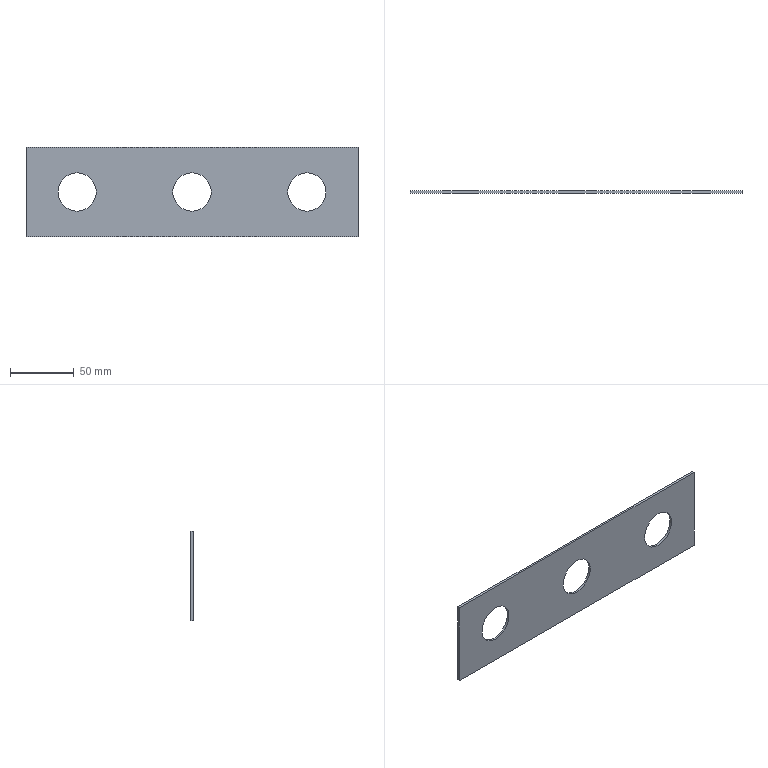Part | STEP file | tutup bawah | 1 solid | 12 faces | box 260 x 1.8 x 70 mm | volume 28943 mm3 | cylinder 6 | plane 6 | commonest cylinder face diameters 30 x6
STEP:
#1=CARTESIAN_POINT('',(0.,0.,0.));
#2=DIRECTION('',(0.,0.,1.));
#3=DIRECTION('',(1.,0.,0.));
#4=AXIS2_PLACEMENT_3D('',#1,#2,#3);
#5=CARTESIAN_POINT('',(90.,1.8,-15.));
#6=VERTEX_POINT('',#5);
#7=CARTESIAN_POINT('',(90.,0.,-15.));
#8=VERTEX_POINT('',#7);
#9=CARTESIAN_POINT('',(90.,1.8,-15.));
#10=DIRECTION('',(0.,-1.,0.));
#11=VECTOR('',#10,1.);
#12=LINE('',#9,#11);
#13=CARTESIAN_POINT('',(90.,1.8,0.));
#14=DIRECTION('',(0.,-1.,0.));
#15=DIRECTION('',(0.,0.,-1.));
#16=AXIS2_PLACEMENT_3D('',#13,#14,#15);
#17=CYLINDRICAL_SURFACE('',#16,15.);
#18=CARTESIAN_POINT('',(6.283,0.));
#19=DIRECTION('',(0.,1.));
#20=VECTOR('',#19,1.);
#21=LINE('',#18,#20);
#22=(GEOMETRIC_REPRESENTATION_CONTEXT(2)PARAMETRIC_REPRESENTATION_CONTEXT()REPRESENTATION_CONTEXT('',''));
#23=DEFINITIONAL_REPRESENTATION('',(#21),#22);
#24=PCURVE('',#17,#23);
#25=CARTESIAN_POINT('',(90.,1.8,0.));
#26=DIRECTION('',(0.,-1.,0.));
#27=DIRECTION('',(0.,0.,-1.));
#28=AXIS2_PLACEMENT_3D('',#25,#26,#27);
#29=CYLINDRICAL_SURFACE('',#28,15.);
#30=CARTESIAN_POINT('',(0.,0.));
#31=DIRECTION('',(0.,1.));
#32=VECTOR('',#31,1.);
#33=LINE('',#30,#32);
#34=(GEOMETRIC_REPRESENTATION_CONTEXT(2)PARAMETRIC_REPRESENTATION_CONTEXT()REPRESENTATION_CONTEXT('',''));
#35=DEFINITIONAL_REPRESENTATION('',(#33),#34);
#36=PCURVE('',#29,#35);
#37=SURFACE_CURVE('',#12,(#24,#36),.PCURVE_S1.);
#38=EDGE_CURVE('',#6,#8,#37,.T.);
#39=ORIENTED_EDGE('',*,*,#38,.T.);
#40=CARTESIAN_POINT('',(90.,0.,15.));
#41=VERTEX_POINT('',#40);
#42=CARTESIAN_POINT('',(90.,0.,0.));
#43=DIRECTION('',(0.,1.,0.));
#44=DIRECTION('',(0.,0.,-1.));
#45=AXIS2_PLACEMENT_3D('',#42,#43,#44);
#46=CIRCLE('',#45,15.);
#47=CARTESIAN_POINT('',(6.283,1.8));
#48=DIRECTION('',(-1.,0.));
#49=VECTOR('',#48,1.);
#50=LINE('',#47,#49);
#51=(GEOMETRIC_REPRESENTATION_CONTEXT(2)PARAMETRIC_REPRESENTATION_CONTEXT()REPRESENTATION_CONTEXT('',''));
#52=DEFINITIONAL_REPRESENTATION('',(#50),#51);
#53=PCURVE('',#17,#52);
#54=CARTESIAN_POINT('',(130.,0.,35.));
#55=DIRECTION('',(0.,1.,0.));
#56=DIRECTION('',(0.,0.,1.));
#57=AXIS2_PLACEMENT_3D('',#54,#55,#56);
#58=PLANE('',#57);
#59=CARTESIAN_POINT('',(-35.,-40.));
#60=DIRECTION('',(-1.,0.));
#61=AXIS2_PLACEMENT_2D('',#59,#60);
#62=CIRCLE('',#61,15.);
#63=(GEOMETRIC_REPRESENTATION_CONTEXT(2)PARAMETRIC_REPRESENTATION_CONTEXT()REPRESENTATION_CONTEXT('',''));
#64=DEFINITIONAL_REPRESENTATION('',(#62),#63);
#65=PCURVE('',#58,#64);
#66=SURFACE_CURVE('',#46,(#53,#65),.PCURVE_S1.);
#67=EDGE_CURVE('',#8,#41,#66,.T.);
#68=ORIENTED_EDGE('',*,*,#67,.T.);
#69=CARTESIAN_POINT('',(90.,1.8,15.));
#70=VERTEX_POINT('',#69);
#71=CARTESIAN_POINT('',(90.,1.8,15.));
#72=DIRECTION('',(0.,-1.,0.));
#73=VECTOR('',#72,1.);
#74=LINE('',#71,#73);
#75=CARTESIAN_POINT('',(3.142,0.));
#76=DIRECTION('',(0.,1.));
#77=VECTOR('',#76,1.);
#78=LINE('',#75,#77);
#79=(GEOMETRIC_REPRESENTATION_CONTEXT(2)PARAMETRIC_REPRESENTATION_CONTEXT()REPRESENTATION_CONTEXT('',''));
#80=DEFINITIONAL_REPRESENTATION('',(#78),#79);
#81=PCURVE('',#17,#80);
#82=CARTESIAN_POINT('',(3.142,0.));
#83=DIRECTION('',(0.,1.));
#84=VECTOR('',#83,1.);
#85=LINE('',#82,#84);
#86=(GEOMETRIC_REPRESENTATION_CONTEXT(2)PARAMETRIC_REPRESENTATION_CONTEXT()REPRESENTATION_CONTEXT('',''));
#87=DEFINITIONAL_REPRESENTATION('',(#85),#86);
#88=PCURVE('',#29,#87);
#89=SURFACE_CURVE('',#74,(#81,#88),.PCURVE_S1.);
#90=EDGE_CURVE('',#70,#41,#89,.T.);
#91=ORIENTED_EDGE('',*,*,#90,.F.);
#92=CARTESIAN_POINT('',(90.,1.8,0.));
#93=DIRECTION('',(0.,1.,0.));
#94=DIRECTION('',(0.,0.,-1.));
#95=AXIS2_PLACEMENT_3D('',#92,#93,#94);
#96=CIRCLE('',#95,15.);
#97=CARTESIAN_POINT('',(6.283,0.));
#98=DIRECTION('',(-1.,0.));
#99=VECTOR('',#98,1.);
#100=LINE('',#97,#99);
#101=(GEOMETRIC_REPRESENTATION_CONTEXT(2)PARAMETRIC_REPRESENTATION_CONTEXT()REPRESENTATION_CONTEXT('',''));
#102=DEFINITIONAL_REPRESENTATION('',(#100),#101);
#103=PCURVE('',#17,#102);
#104=CARTESIAN_POINT('',(130.,1.8,35.));
#105=DIRECTION('',(0.,1.,0.));
#106=DIRECTION('',(0.,0.,1.));
#107=AXIS2_PLACEMENT_3D('',#104,#105,#106);
#108=PLANE('',#107);
#109=CARTESIAN_POINT('',(-35.,-40.));
#110=DIRECTION('',(-1.,0.));
#111=AXIS2_PLACEMENT_2D('',#109,#110);
#112=CIRCLE('',#111,15.);
#113=(GEOMETRIC_REPRESENTATION_CONTEXT(2)PARAMETRIC_REPRESENTATION_CONTEXT()REPRESENTATION_CONTEXT('',''));
#114=DEFINITIONAL_REPRESENTATION('',(#112),#113);
#115=PCURVE('',#108,#114);
#116=SURFACE_CURVE('',#96,(#103,#115),.PCURVE_S1.);
#117=EDGE_CURVE('',#6,#70,#116,.T.);
#118=ORIENTED_EDGE('',*,*,#117,.F.);
#119=EDGE_LOOP('',(#39,#68,#91,#118));
#120=FACE_BOUND('',#119,.F.);
#121=ADVANCED_FACE('',(#120),#17,.F.);
#122=CARTESIAN_POINT('',(0.,1.8,-15.));
#123=VERTEX_POINT('',#122);
#124=CARTESIAN_POINT('',(0.,0.,-15.));
#125=VERTEX_POINT('',#124);
#126=CARTESIAN_POINT('',(0.,1.8,-15.));
#127=DIRECTION('',(0.,-1.,0.));
#128=VECTOR('',#127,1.);
#129=LINE('',#126,#128);
#130=CARTESIAN_POINT('',(0.,1.8,0.));
#131=DIRECTION('',(0.,-1.,0.));
#132=DIRECTION('',(0.,0.,-1.));
#133=AXIS2_PLACEMENT_3D('',#130,#131,#132);
#134=CYLINDRICAL_SURFACE('',#133,15.);
#135=CARTESIAN_POINT('',(6.283,0.));
#136=DIRECTION('',(0.,1.));
#137=VECTOR('',#136,1.);
#138=LINE('',#135,#137);
#139=(GEOMETRIC_REPRESENTATION_CONTEXT(2)PARAMETRIC_REPRESENTATION_CONTEXT()REPRESENTATION_CONTEXT('',''));
#140=DEFINITIONAL_REPRESENTATION('',(#138),#139);
#141=PCURVE('',#134,#140);
#142=CARTESIAN_POINT('',(0.,1.8,0.));
#143=DIRECTION('',(0.,-1.,0.));
#144=DIRECTION('',(0.,0.,-1.));
#145=AXIS2_PLACEMENT_3D('',#142,#143,#144);
#146=CYLINDRICAL_SURFACE('',#145,15.);
#147=CARTESIAN_POINT('',(0.,0.));
#148=DIRECTION('',(0.,1.));
#149=VECTOR('',#148,1.);
#150=LINE('',#147,#149);
#151=(GEOMETRIC_REPRESENTATION_CONTEXT(2)PARAMETRIC_REPRESENTATION_CONTEXT()REPRESENTATION_CONTEXT('',''));
#152=DEFINITIONAL_REPRESENTATION('',(#150),#151);
#153=PCURVE('',#146,#152);
#154=SURFACE_CURVE('',#129,(#141,#153),.PCURVE_S1.);
#155=EDGE_CURVE('',#123,#125,#154,.T.);
#156=ORIENTED_EDGE('',*,*,#155,.T.);
#157=CARTESIAN_POINT('',(0.,0.,15.));
#158=VERTEX_POINT('',#157);
#159=CARTESIAN_POINT('',(0.,0.,0.));
#160=DIRECTION('',(0.,1.,0.));
#161=DIRECTION('',(0.,0.,1.));
#162=AXIS2_PLACEMENT_3D('',#159,#160,#161);
#163=CIRCLE('',#162,15.);
#164=CARTESIAN_POINT('',(9.425,1.8));
#165=DIRECTION('',(-1.,0.));
#166=VECTOR('',#165,1.);
#167=LINE('',#164,#166);
#168=(GEOMETRIC_REPRESENTATION_CONTEXT(2)PARAMETRIC_REPRESENTATION_CONTEXT()REPRESENTATION_CONTEXT('',''));
#169=DEFINITIONAL_REPRESENTATION('',(#167),#168);
#170=PCURVE('',#134,#169);
#171=CARTESIAN_POINT('',(-35.,-130.));
#172=DIRECTION('',(1.,0.));
#173=AXIS2_PLACEMENT_2D('',#171,#172);
#174=CIRCLE('',#173,15.);
#175=(GEOMETRIC_REPRESENTATION_CONTEXT(2)PARAMETRIC_REPRESENTATION_CONTEXT()REPRESENTATION_CONTEXT('',''));
#176=DEFINITIONAL_REPRESENTATION('',(#174),#175);
#177=PCURVE('',#58,#176);
#178=SURFACE_CURVE('',#163,(#170,#177),.PCURVE_S1.);
#179=EDGE_CURVE('',#125,#158,#178,.T.);
#180=ORIENTED_EDGE('',*,*,#179,.T.);
#181=CARTESIAN_POINT('',(0.,1.8,15.));
#182=VERTEX_POINT('',#181);
#183=CARTESIAN_POINT('',(0.,1.8,15.));
#184=DIRECTION('',(0.,-1.,0.));
#185=VECTOR('',#184,1.);
#186=LINE('',#183,#185);
#187=CARTESIAN_POINT('',(3.142,0.));
#188=DIRECTION('',(0.,1.));
#189=VECTOR('',#188,1.);
#190=LINE('',#187,#189);
#191=(GEOMETRIC_REPRESENTATION_CONTEXT(2)PARAMETRIC_REPRESENTATION_CONTEXT()REPRESENTATION_CONTEXT('',''));
#192=DEFINITIONAL_REPRESENTATION('',(#190),#191);
#193=PCURVE('',#134,#192);
#194=CARTESIAN_POINT('',(3.142,0.));
#195=DIRECTION('',(0.,1.));
#196=VECTOR('',#195,1.);
#197=LINE('',#194,#196);
#198=(GEOMETRIC_REPRESENTATION_CONTEXT(2)PARAMETRIC_REPRESENTATION_CONTEXT()REPRESENTATION_CONTEXT('',''));
#199=DEFINITIONAL_REPRESENTATION('',(#197),#198);
#200=PCURVE('',#146,#199);
#201=SURFACE_CURVE('',#186,(#193,#200),.PCURVE_S1.);
#202=EDGE_CURVE('',#182,#158,#201,.T.);
#203=ORIENTED_EDGE('',*,*,#202,.F.);
#204=CARTESIAN_POINT('',(0.,1.8,0.));
#205=DIRECTION('',(0.,1.,0.));
#206=DIRECTION('',(0.,0.,1.));
#207=AXIS2_PLACEMENT_3D('',#204,#205,#206);
#208=CIRCLE('',#207,15.);
#209=CARTESIAN_POINT('',(9.425,0.));
#210=DIRECTION('',(-1.,0.));
#211=VECTOR('',#210,1.);
#212=LINE('',#209,#211);
#213=(GEOMETRIC_REPRESENTATION_CONTEXT(2)PARAMETRIC_REPRESENTATION_CONTEXT()REPRESENTATION_CONTEXT('',''));
#214=DEFINITIONAL_REPRESENTATION('',(#212),#213);
#215=PCURVE('',#134,#214);
#216=CARTESIAN_POINT('',(-35.,-130.));
#217=DIRECTION('',(1.,0.));
#218=AXIS2_PLACEMENT_2D('',#216,#217);
#219=CIRCLE('',#218,15.);
#220=(GEOMETRIC_REPRESENTATION_CONTEXT(2)PARAMETRIC_REPRESENTATION_CONTEXT()REPRESENTATION_CONTEXT('',''));
#221=DEFINITIONAL_REPRESENTATION('',(#219),#220);
#222=PCURVE('',#108,#221);
#223=SURFACE_CURVE('',#208,(#215,#222),.PCURVE_S1.);
#224=EDGE_CURVE('',#123,#182,#223,.T.);
#225=ORIENTED_EDGE('',*,*,#224,.F.);
#226=EDGE_LOOP('',(#156,#180,#203,#225));
#227=FACE_BOUND('',#226,.F.);
#228=ADVANCED_FACE('',(#227),#134,.F.);
#229=CARTESIAN_POINT('',(-90.,1.8,-15.));
#230=VERTEX_POINT('',#229);
#231=CARTESIAN_POINT('',(-90.,0.,-15.));
#232=VERTEX_POINT('',#231);
#233=CARTESIAN_POINT('',(-90.,1.8,-15.));
#234=DIRECTION('',(0.,-1.,0.));
#235=VECTOR('',#234,1.);
#236=LINE('',#233,#235);
#237=CARTESIAN_POINT('',(-90.,1.8,0.));
#238=DIRECTION('',(0.,-1.,0.));
#239=DIRECTION('',(0.,0.,-1.));
#240=AXIS2_PLACEMENT_3D('',#237,#238,#239);
#241=CYLINDRICAL_SURFACE('',#240,15.);
#242=CARTESIAN_POINT('',(6.283,0.));
#243=DIRECTION('',(0.,1.));
#244=VECTOR('',#243,1.);
#245=LINE('',#242,#244);
#246=(GEOMETRIC_REPRESENTATION_CONTEXT(2)PARAMETRIC_REPRESENTATION_CONTEXT()REPRESENTATION_CONTEXT('',''));
#247=DEFINITIONAL_REPRESENTATION('',(#245),#246);
#248=PCURVE('',#241,#247);
#249=CARTESIAN_POINT('',(-90.,1.8,0.));
#250=DIRECTION('',(0.,-1.,0.));
#251=DIRECTION('',(0.,0.,-1.));
#252=AXIS2_PLACEMENT_3D('',#249,#250,#251);
#253=CYLINDRICAL_SURFACE('',#252,15.);
#254=CARTESIAN_POINT('',(0.,0.));
#255=DIRECTION('',(0.,1.));
#256=VECTOR('',#255,1.);
#257=LINE('',#254,#256);
#258=(GEOMETRIC_REPRESENTATION_CONTEXT(2)PARAMETRIC_REPRESENTATION_CONTEXT()REPRESENTATION_CONTEXT('',''));
#259=DEFINITIONAL_REPRESENTATION('',(#257),#258);
#260=PCURVE('',#253,#259);
#261=SURFACE_CURVE('',#236,(#248,#260),.PCURVE_S1.);
#262=EDGE_CURVE('',#230,#232,#261,.T.);
#263=ORIENTED_EDGE('',*,*,#262,.T.);
#264=CARTESIAN_POINT('',(-90.,0.,15.));
#265=VERTEX_POINT('',#264);
#266=CARTESIAN_POINT('',(-90.,0.,0.));
#267=DIRECTION('',(0.,1.,0.));
#268=DIRECTION('',(0.,0.,1.));
#269=AXIS2_PLACEMENT_3D('',#266,#267,#268);
#270=CIRCLE('',#269,15.);
#271=CARTESIAN_POINT('',(9.425,1.8));
#272=DIRECTION('',(-1.,0.));
#273=VECTOR('',#272,1.);
#274=LINE('',#271,#273);
#275=(GEOMETRIC_REPRESENTATION_CONTEXT(2)PARAMETRIC_REPRESENTATION_CONTEXT()REPRESENTATION_CONTEXT('',''));
#276=DEFINITIONAL_REPRESENTATION('',(#274),#275);
#277=PCURVE('',#241,#276);
#278=CARTESIAN_POINT('',(-35.,-220.));
#279=DIRECTION('',(1.,0.));
#280=AXIS2_PLACEMENT_2D('',#278,#279);
#281=CIRCLE('',#280,15.);
#282=(GEOMETRIC_REPRESENTATION_CONTEXT(2)PARAMETRIC_REPRESENTATION_CONTEXT()REPRESENTATION_CONTEXT('',''));
#283=DEFINITIONAL_REPRESENTATION('',(#281),#282);
#284=PCURVE('',#58,#283);
#285=SURFACE_CURVE('',#270,(#277,#284),.PCURVE_S1.);
#286=EDGE_CURVE('',#232,#265,#285,.T.);
#287=ORIENTED_EDGE('',*,*,#286,.T.);
#288=CARTESIAN_POINT('',(-90.,1.8,15.));
#289=VERTEX_POINT('',#288);
#290=CARTESIAN_POINT('',(-90.,1.8,15.));
#291=DIRECTION('',(0.,-1.,0.));
#292=VECTOR('',#291,1.);
#293=LINE('',#290,#292);
#294=CARTESIAN_POINT('',(3.142,0.));
#295=DIRECTION('',(0.,1.));
#296=VECTOR('',#295,1.);
#297=LINE('',#294,#296);
#298=(GEOMETRIC_REPRESENTATION_CONTEXT(2)PARAMETRIC_REPRESENTATION_CONTEXT()REPRESENTATION_CONTEXT('',''));
#299=DEFINITIONAL_REPRESENTATION('',(#297),#298);
#300=PCURVE('',#241,#299);
#301=CARTESIAN_POINT('',(3.142,0.));
#302=DIRECTION('',(0.,1.));
#303=VECTOR('',#302,1.);
#304=LINE('',#301,#303);
#305=(GEOMETRIC_REPRESENTATION_CONTEXT(2)PARAMETRIC_REPRESENTATION_CONTEXT()REPRESENTATION_CONTEXT('',''));
#306=DEFINITIONAL_REPRESENTATION('',(#304),#305);
#307=PCURVE('',#253,#306);
#308=SURFACE_CURVE('',#293,(#300,#307),.PCURVE_S1.);
#309=EDGE_CURVE('',#289,#265,#308,.T.);
#310=ORIENTED_EDGE('',*,*,#309,.F.);
#311=CARTESIAN_POINT('',(-90.,1.8,0.));
#312=DIRECTION('',(0.,1.,0.));
#313=DIRECTION('',(0.,0.,1.));
#314=AXIS2_PLACEMENT_3D('',#311,#312,#313);
#315=CIRCLE('',#314,15.);
#316=CARTESIAN_POINT('',(9.425,0.));
#317=DIRECTION('',(-1.,0.));
#318=VECTOR('',#317,1.);
#319=LINE('',#316,#318);
#320=(GEOMETRIC_REPRESENTATION_CONTEXT(2)PARAMETRIC_REPRESENTATION_CONTEXT()REPRESENTATION_CONTEXT('',''));
#321=DEFINITIONAL_REPRESENTATION('',(#319),#320);
#322=PCURVE('',#241,#321);
#323=CARTESIAN_POINT('',(-35.,-220.));
#324=DIRECTION('',(1.,0.));
#325=AXIS2_PLACEMENT_2D('',#323,#324);
#326=CIRCLE('',#325,15.);
#327=(GEOMETRIC_REPRESENTATION_CONTEXT(2)PARAMETRIC_REPRESENTATION_CONTEXT()REPRESENTATION_CONTEXT('',''));
#328=DEFINITIONAL_REPRESENTATION('',(#326),#327);
#329=PCURVE('',#108,#328);
#330=SURFACE_CURVE('',#315,(#322,#329),.PCURVE_S1.);
#331=EDGE_CURVE('',#230,#289,#330,.T.);
#332=ORIENTED_EDGE('',*,*,#331,.F.);
#333=EDGE_LOOP('',(#263,#287,#310,#332));
#334=FACE_BOUND('',#333,.F.);
#335=ADVANCED_FACE('',(#334),#241,.F.);
#336=ORIENTED_EDGE('',*,*,#224,.F.);
#337=CARTESIAN_POINT('',(0.,1.8,0.));
#338=DIRECTION('',(0.,1.,0.));
#339=DIRECTION('',(0.,0.,1.));
#340=AXIS2_PLACEMENT_3D('',#337,#338,#339);
#341=CIRCLE('',#340,15.);
#342=CARTESIAN_POINT('',(-35.,-130.));
#343=DIRECTION('',(1.,0.));
#344=AXIS2_PLACEMENT_2D('',#342,#343);
#345=CIRCLE('',#344,15.);
#346=(GEOMETRIC_REPRESENTATION_CONTEXT(2)PARAMETRIC_REPRESENTATION_CONTEXT()REPRESENTATION_CONTEXT('',''));
#347=DEFINITIONAL_REPRESENTATION('',(#345),#346);
#348=PCURVE('',#108,#347);
#349=CARTESIAN_POINT('',(3.142,0.));
#350=DIRECTION('',(-1.,0.));
#351=VECTOR('',#350,1.);
#352=LINE('',#349,#351);
#353=(GEOMETRIC_REPRESENTATION_CONTEXT(2)PARAMETRIC_REPRESENTATION_CONTEXT()REPRESENTATION_CONTEXT('',''));
#354=DEFINITIONAL_REPRESENTATION('',(#352),#353);
#355=PCURVE('',#146,#354);
#356=SURFACE_CURVE('',#341,(#348,#355),.PCURVE_S1.);
#357=EDGE_CURVE('',#182,#123,#356,.T.);
#358=ORIENTED_EDGE('',*,*,#357,.F.);
#359=EDGE_LOOP('',(#336,#358));
#360=FACE_BOUND('',#359,.T.);
#361=CARTESIAN_POINT('',(130.,1.8,35.));
#362=VERTEX_POINT('',#361);
#363=CARTESIAN_POINT('',(130.,1.8,-35.));
#364=VERTEX_POINT('',#363);
#365=CARTESIAN_POINT('',(130.,1.8,-35.));
#366=DIRECTION('',(0.,0.,-1.));
#367=VECTOR('',#366,1.);
#368=LINE('',#365,#367);
#369=CARTESIAN_POINT('',(-70.,0.));
#370=DIRECTION('',(-1.,0.));
#371=VECTOR('',#370,1.);
#372=LINE('',#369,#371);
#373=(GEOMETRIC_REPRESENTATION_CONTEXT(2)PARAMETRIC_REPRESENTATION_CONTEXT()REPRESENTATION_CONTEXT('',''));
#374=DEFINITIONAL_REPRESENTATION('',(#372),#373);
#375=PCURVE('',#108,#374);
#376=CARTESIAN_POINT('',(130.,1.8,-35.));
#377=DIRECTION('',(-1.,0.,0.));
#378=DIRECTION('',(0.,0.,1.));
#379=AXIS2_PLACEMENT_3D('',#376,#377,#378);
#380=PLANE('',#379);
#381=CARTESIAN_POINT('',(0.,0.));
#382=DIRECTION('',(-1.,0.));
#383=VECTOR('',#382,1.);
#384=LINE('',#381,#383);
#385=(GEOMETRIC_REPRESENTATION_CONTEXT(2)PARAMETRIC_REPRESENTATION_CONTEXT()REPRESENTATION_CONTEXT('',''));
#386=DEFINITIONAL_REPRESENTATION('',(#384),#385);
#387=PCURVE('',#380,#386);
#388=SURFACE_CURVE('',#368,(#375,#387),.PCURVE_S1.);
#389=EDGE_CURVE('',#362,#364,#388,.T.);
#390=ORIENTED_EDGE('',*,*,#389,.T.);
#391=CARTESIAN_POINT('',(-130.,1.8,-35.));
#392=VERTEX_POINT('',#391);
#393=CARTESIAN_POINT('',(-130.,1.8,-35.));
#394=DIRECTION('',(-1.,0.,0.));
#395=VECTOR('',#394,1.);
#396=LINE('',#393,#395);
#397=CARTESIAN_POINT('',(-70.,-260.));
#398=DIRECTION('',(0.,-1.));
#399=VECTOR('',#398,1.);
#400=LINE('',#397,#399);
#401=(GEOMETRIC_REPRESENTATION_CONTEXT(2)PARAMETRIC_REPRESENTATION_CONTEXT()REPRESENTATION_CONTEXT('',''));
#402=DEFINITIONAL_REPRESENTATION('',(#400),#401);
#403=PCURVE('',#108,#402);
#404=CARTESIAN_POINT('',(-130.,1.8,-35.));
#405=DIRECTION('',(0.,0.,1.));
#406=DIRECTION('',(1.,0.,0.));
#407=AXIS2_PLACEMENT_3D('',#404,#405,#406);
#408=PLANE('',#407);
#409=CARTESIAN_POINT('',(0.,0.));
#410=DIRECTION('',(-1.,0.));
#411=VECTOR('',#410,1.);
#412=LINE('',#409,#411);
#413=(GEOMETRIC_REPRESENTATION_CONTEXT(2)PARAMETRIC_REPRESENTATION_CONTEXT()REPRESENTATION_CONTEXT('',''));
#414=DEFINITIONAL_REPRESENTATION('',(#412),#413);
#415=PCURVE('',#408,#414);
#416=SURFACE_CURVE('',#396,(#403,#415),.PCURVE_S1.);
#417=EDGE_CURVE('',#364,#392,#416,.T.);
#418=ORIENTED_EDGE('',*,*,#417,.T.);
#419=CARTESIAN_POINT('',(-130.,1.8,35.));
#420=VERTEX_POINT('',#419);
#421=CARTESIAN_POINT('',(-130.,1.8,-35.));
#422=DIRECTION('',(0.,0.,1.));
#423=VECTOR('',#422,1.);
#424=LINE('',#421,#423);
#425=CARTESIAN_POINT('',(-70.,-260.));
#426=DIRECTION('',(1.,0.));
#427=VECTOR('',#426,1.);
#428=LINE('',#425,#427);
#429=(GEOMETRIC_REPRESENTATION_CONTEXT(2)PARAMETRIC_REPRESENTATION_CONTEXT()REPRESENTATION_CONTEXT('',''));
#430=DEFINITIONAL_REPRESENTATION('',(#428),#429);
#431=PCURVE('',#108,#430);
#432=CARTESIAN_POINT('',(-130.,1.8,-35.));
#433=DIRECTION('',(1.,0.,0.));
#434=DIRECTION('',(0.,0.,-1.));
#435=AXIS2_PLACEMENT_3D('',#432,#433,#434);
#436=PLANE('',#435);
#437=CARTESIAN_POINT('',(0.,0.));
#438=DIRECTION('',(-1.,0.));
#439=VECTOR('',#438,1.);
#440=LINE('',#437,#439);
#441=(GEOMETRIC_REPRESENTATION_CONTEXT(2)PARAMETRIC_REPRESENTATION_CONTEXT()REPRESENTATION_CONTEXT('',''));
#442=DEFINITIONAL_REPRESENTATION('',(#440),#441);
#443=PCURVE('',#436,#442);
#444=SURFACE_CURVE('',#424,(#431,#443),.PCURVE_S1.);
#445=EDGE_CURVE('',#392,#420,#444,.T.);
#446=ORIENTED_EDGE('',*,*,#445,.T.);
#447=CARTESIAN_POINT('',(-130.,1.8,35.));
#448=DIRECTION('',(1.,0.,0.));
#449=VECTOR('',#448,1.);
#450=LINE('',#447,#449);
#451=CARTESIAN_POINT('',(0.,-260.));
#452=DIRECTION('',(0.,1.));
#453=VECTOR('',#452,1.);
#454=LINE('',#451,#453);
#455=(GEOMETRIC_REPRESENTATION_CONTEXT(2)PARAMETRIC_REPRESENTATION_CONTEXT()REPRESENTATION_CONTEXT('',''));
#456=DEFINITIONAL_REPRESENTATION('',(#454),#455);
#457=PCURVE('',#108,#456);
#458=CARTESIAN_POINT('',(-130.,1.8,35.));
#459=DIRECTION('',(0.,0.,-1.));
#460=DIRECTION('',(-1.,0.,0.));
#461=AXIS2_PLACEMENT_3D('',#458,#459,#460);
#462=PLANE('',#461);
#463=CARTESIAN_POINT('',(0.,0.));
#464=DIRECTION('',(-1.,0.));
#465=VECTOR('',#464,1.);
#466=LINE('',#463,#465);
#467=(GEOMETRIC_REPRESENTATION_CONTEXT(2)PARAMETRIC_REPRESENTATION_CONTEXT()REPRESENTATION_CONTEXT('',''));
#468=DEFINITIONAL_REPRESENTATION('',(#466),#467);
#469=PCURVE('',#462,#468);
#470=SURFACE_CURVE('',#450,(#457,#469),.PCURVE_S1.);
#471=EDGE_CURVE('',#420,#362,#470,.T.);
#472=ORIENTED_EDGE('',*,*,#471,.T.);
#473=EDGE_LOOP('',(#390,#418,#446,#472));
#474=FACE_BOUND('',#473,.T.);
#475=ORIENTED_EDGE('',*,*,#331,.F.);
#476=CARTESIAN_POINT('',(-90.,1.8,0.));
#477=DIRECTION('',(0.,1.,0.));
#478=DIRECTION('',(0.,0.,1.));
#479=AXIS2_PLACEMENT_3D('',#476,#477,#478);
#480=CIRCLE('',#479,15.);
#481=CARTESIAN_POINT('',(-35.,-220.));
#482=DIRECTION('',(1.,0.));
#483=AXIS2_PLACEMENT_2D('',#481,#482);
#484=CIRCLE('',#483,15.);
#485=(GEOMETRIC_REPRESENTATION_CONTEXT(2)PARAMETRIC_REPRESENTATION_CONTEXT()REPRESENTATION_CONTEXT('',''));
#486=DEFINITIONAL_REPRESENTATION('',(#484),#485);
#487=PCURVE('',#108,#486);
#488=CARTESIAN_POINT('',(3.142,0.));
#489=DIRECTION('',(-1.,0.));
#490=VECTOR('',#489,1.);
#491=LINE('',#488,#490);
#492=(GEOMETRIC_REPRESENTATION_CONTEXT(2)PARAMETRIC_REPRESENTATION_CONTEXT()REPRESENTATION_CONTEXT('',''));
#493=DEFINITIONAL_REPRESENTATION('',(#491),#492);
#494=PCURVE('',#253,#493);
#495=SURFACE_CURVE('',#480,(#487,#494),.PCURVE_S1.);
#496=EDGE_CURVE('',#289,#230,#495,.T.);
#497=ORIENTED_EDGE('',*,*,#496,.F.);
#498=EDGE_LOOP('',(#475,#497));
#499=FACE_BOUND('',#498,.T.);
#500=ORIENTED_EDGE('',*,*,#117,.F.);
#501=CARTESIAN_POINT('',(90.,1.8,0.));
#502=DIRECTION('',(0.,1.,0.));
#503=DIRECTION('',(0.,0.,-1.));
#504=AXIS2_PLACEMENT_3D('',#501,#502,#503);
#505=CIRCLE('',#504,15.);
#506=CARTESIAN_POINT('',(-35.,-40.));
#507=DIRECTION('',(-1.,0.));
#508=AXIS2_PLACEMENT_2D('',#506,#507);
#509=CIRCLE('',#508,15.);
#510=(GEOMETRIC_REPRESENTATION_CONTEXT(2)PARAMETRIC_REPRESENTATION_CONTEXT()REPRESENTATION_CONTEXT('',''));
#511=DEFINITIONAL_REPRESENTATION('',(#509),#510);
#512=PCURVE('',#108,#511);
#513=CARTESIAN_POINT('',(6.283,0.));
#514=DIRECTION('',(-1.,0.));
#515=VECTOR('',#514,1.);
#516=LINE('',#513,#515);
#517=(GEOMETRIC_REPRESENTATION_CONTEXT(2)PARAMETRIC_REPRESENTATION_CONTEXT()REPRESENTATION_CONTEXT('',''));
#518=DEFINITIONAL_REPRESENTATION('',(#516),#517);
#519=PCURVE('',#29,#518);
#520=SURFACE_CURVE('',#505,(#512,#519),.PCURVE_S1.);
#521=EDGE_CURVE('',#70,#6,#520,.T.);
#522=ORIENTED_EDGE('',*,*,#521,.F.);
#523=EDGE_LOOP('',(#500,#522));
#524=FACE_BOUND('',#523,.T.);
#525=ADVANCED_FACE('',(#360,#474,#499,#524),#108,.T.);
#526=ORIENTED_EDGE('',*,*,#179,.T.);
#527=CARTESIAN_POINT('',(0.,0.,0.));
#528=DIRECTION('',(0.,1.,0.));
#529=DIRECTION('',(0.,0.,1.));
#530=AXIS2_PLACEMENT_3D('',#527,#528,#529);
#531=CIRCLE('',#530,15.);
#532=CARTESIAN_POINT('',(-35.,-130.));
#533=DIRECTION('',(1.,0.));
#534=AXIS2_PLACEMENT_2D('',#532,#533);
#535=CIRCLE('',#534,15.);
#536=(GEOMETRIC_REPRESENTATION_CONTEXT(2)PARAMETRIC_REPRESENTATION_CONTEXT()REPRESENTATION_CONTEXT('',''));
#537=DEFINITIONAL_REPRESENTATION('',(#535),#536);
#538=PCURVE('',#58,#537);
#539=CARTESIAN_POINT('',(3.142,1.8));
#540=DIRECTION('',(-1.,0.));
#541=VECTOR('',#540,1.);
#542=LINE('',#539,#541);
#543=(GEOMETRIC_REPRESENTATION_CONTEXT(2)PARAMETRIC_REPRESENTATION_CONTEXT()REPRESENTATION_CONTEXT('',''));
#544=DEFINITIONAL_REPRESENTATION('',(#542),#543);
#545=PCURVE('',#146,#544);
#546=SURFACE_CURVE('',#531,(#538,#545),.PCURVE_S1.);
#547=EDGE_CURVE('',#158,#125,#546,.T.);
#548=ORIENTED_EDGE('',*,*,#547,.T.);
#549=EDGE_LOOP('',(#526,#548));
#550=FACE_BOUND('',#549,.T.);
#551=CARTESIAN_POINT('',(130.,0.,35.));
#552=VERTEX_POINT('',#551);
#553=CARTESIAN_POINT('',(130.,0.,-35.));
#554=VERTEX_POINT('',#553);
#555=CARTESIAN_POINT('',(130.,0.,-35.));
#556=DIRECTION('',(0.,0.,-1.));
#557=VECTOR('',#556,1.);
#558=LINE('',#555,#557);
#559=CARTESIAN_POINT('',(-70.,0.));
#560=DIRECTION('',(-1.,0.));
#561=VECTOR('',#560,1.);
#562=LINE('',#559,#561);
#563=(GEOMETRIC_REPRESENTATION_CONTEXT(2)PARAMETRIC_REPRESENTATION_CONTEXT()REPRESENTATION_CONTEXT('',''));
#564=DEFINITIONAL_REPRESENTATION('',(#562),#563);
#565=PCURVE('',#58,#564);
#566=CARTESIAN_POINT('',(0.,-1.8));
#567=DIRECTION('',(-1.,0.));
#568=VECTOR('',#567,1.);
#569=LINE('',#566,#568);
#570=(GEOMETRIC_REPRESENTATION_CONTEXT(2)PARAMETRIC_REPRESENTATION_CONTEXT()REPRESENTATION_CONTEXT('',''));
#571=DEFINITIONAL_REPRESENTATION('',(#569),#570);
#572=PCURVE('',#380,#571);
#573=SURFACE_CURVE('',#558,(#565,#572),.PCURVE_S1.);
#574=EDGE_CURVE('',#552,#554,#573,.T.);
#575=ORIENTED_EDGE('',*,*,#574,.F.);
#576=CARTESIAN_POINT('',(-130.,0.,35.));
#577=VERTEX_POINT('',#576);
#578=CARTESIAN_POINT('',(-130.,0.,35.));
#579=DIRECTION('',(1.,0.,0.));
#580=VECTOR('',#579,1.);
#581=LINE('',#578,#580);
#582=CARTESIAN_POINT('',(0.,-260.));
#583=DIRECTION('',(0.,1.));
#584=VECTOR('',#583,1.);
#585=LINE('',#582,#584);
#586=(GEOMETRIC_REPRESENTATION_CONTEXT(2)PARAMETRIC_REPRESENTATION_CONTEXT()REPRESENTATION_CONTEXT('',''));
#587=DEFINITIONAL_REPRESENTATION('',(#585),#586);
#588=PCURVE('',#58,#587);
#589=CARTESIAN_POINT('',(0.,-1.8));
#590=DIRECTION('',(-1.,0.));
#591=VECTOR('',#590,1.);
#592=LINE('',#589,#591);
#593=(GEOMETRIC_REPRESENTATION_CONTEXT(2)PARAMETRIC_REPRESENTATION_CONTEXT()REPRESENTATION_CONTEXT('',''));
#594=DEFINITIONAL_REPRESENTATION('',(#592),#593);
#595=PCURVE('',#462,#594);
#596=SURFACE_CURVE('',#581,(#588,#595),.PCURVE_S1.);
#597=EDGE_CURVE('',#577,#552,#596,.T.);
#598=ORIENTED_EDGE('',*,*,#597,.F.);
#599=CARTESIAN_POINT('',(-130.,0.,-35.));
#600=VERTEX_POINT('',#599);
#601=CARTESIAN_POINT('',(-130.,0.,-35.));
#602=DIRECTION('',(0.,0.,1.));
#603=VECTOR('',#602,1.);
#604=LINE('',#601,#603);
#605=CARTESIAN_POINT('',(-70.,-260.));
#606=DIRECTION('',(1.,0.));
#607=VECTOR('',#606,1.);
#608=LINE('',#605,#607);
#609=(GEOMETRIC_REPRESENTATION_CONTEXT(2)PARAMETRIC_REPRESENTATION_CONTEXT()REPRESENTATION_CONTEXT('',''));
#610=DEFINITIONAL_REPRESENTATION('',(#608),#609);
#611=PCURVE('',#58,#610);
#612=CARTESIAN_POINT('',(0.,-1.8));
#613=DIRECTION('',(-1.,0.));
#614=VECTOR('',#613,1.);
#615=LINE('',#612,#614);
#616=(GEOMETRIC_REPRESENTATION_CONTEXT(2)PARAMETRIC_REPRESENTATION_CONTEXT()REPRESENTATION_CONTEXT('',''));
#617=DEFINITIONAL_REPRESENTATION('',(#615),#616);
#618=PCURVE('',#436,#617);
#619=SURFACE_CURVE('',#604,(#611,#618),.PCURVE_S1.);
#620=EDGE_CURVE('',#600,#577,#619,.T.);
#621=ORIENTED_EDGE('',*,*,#620,.F.);
#622=CARTESIAN_POINT('',(-130.,0.,-35.));
#623=DIRECTION('',(-1.,0.,0.));
#624=VECTOR('',#623,1.);
#625=LINE('',#622,#624);
#626=CARTESIAN_POINT('',(-70.,-260.));
#627=DIRECTION('',(0.,-1.));
#628=VECTOR('',#627,1.);
#629=LINE('',#626,#628);
#630=(GEOMETRIC_REPRESENTATION_CONTEXT(2)PARAMETRIC_REPRESENTATION_CONTEXT()REPRESENTATION_CONTEXT('',''));
#631=DEFINITIONAL_REPRESENTATION('',(#629),#630);
#632=PCURVE('',#58,#631);
#633=CARTESIAN_POINT('',(0.,-1.8));
#634=DIRECTION('',(-1.,0.));
#635=VECTOR('',#634,1.);
#636=LINE('',#633,#635);
#637=(GEOMETRIC_REPRESENTATION_CONTEXT(2)PARAMETRIC_REPRESENTATION_CONTEXT()REPRESENTATION_CONTEXT('',''));
#638=DEFINITIONAL_REPRESENTATION('',(#636),#637);
#639=PCURVE('',#408,#638);
#640=SURFACE_CURVE('',#625,(#632,#639),.PCURVE_S1.);
#641=EDGE_CURVE('',#554,#600,#640,.T.);
#642=ORIENTED_EDGE('',*,*,#641,.F.);
#643=EDGE_LOOP('',(#575,#598,#621,#642));
#644=FACE_BOUND('',#643,.T.);
#645=ORIENTED_EDGE('',*,*,#286,.T.);
#646=CARTESIAN_POINT('',(-90.,0.,0.));
#647=DIRECTION('',(0.,1.,0.));
#648=DIRECTION('',(0.,0.,1.));
#649=AXIS2_PLACEMENT_3D('',#646,#647,#648);
#650=CIRCLE('',#649,15.);
#651=CARTESIAN_POINT('',(-35.,-220.));
#652=DIRECTION('',(1.,0.));
#653=AXIS2_PLACEMENT_2D('',#651,#652);
#654=CIRCLE('',#653,15.);
#655=(GEOMETRIC_REPRESENTATION_CONTEXT(2)PARAMETRIC_REPRESENTATION_CONTEXT()REPRESENTATION_CONTEXT('',''));
#656=DEFINITIONAL_REPRESENTATION('',(#654),#655);
#657=PCURVE('',#58,#656);
#658=CARTESIAN_POINT('',(3.142,1.8));
#659=DIRECTION('',(-1.,0.));
#660=VECTOR('',#659,1.);
#661=LINE('',#658,#660);
#662=(GEOMETRIC_REPRESENTATION_CONTEXT(2)PARAMETRIC_REPRESENTATION_CONTEXT()REPRESENTATION_CONTEXT('',''));
#663=DEFINITIONAL_REPRESENTATION('',(#661),#662);
#664=PCURVE('',#253,#663);
#665=SURFACE_CURVE('',#650,(#657,#664),.PCURVE_S1.);
#666=EDGE_CURVE('',#265,#232,#665,.T.);
#667=ORIENTED_EDGE('',*,*,#666,.T.);
#668=EDGE_LOOP('',(#645,#667));
#669=FACE_BOUND('',#668,.T.);
#670=ORIENTED_EDGE('',*,*,#67,.T.);
#671=CARTESIAN_POINT('',(90.,0.,0.));
#672=DIRECTION('',(0.,1.,0.));
#673=DIRECTION('',(0.,0.,-1.));
#674=AXIS2_PLACEMENT_3D('',#671,#672,#673);
#675=CIRCLE('',#674,15.);
#676=CARTESIAN_POINT('',(-35.,-40.));
#677=DIRECTION('',(-1.,0.));
#678=AXIS2_PLACEMENT_2D('',#676,#677);
#679=CIRCLE('',#678,15.);
#680=(GEOMETRIC_REPRESENTATION_CONTEXT(2)PARAMETRIC_REPRESENTATION_CONTEXT()REPRESENTATION_CONTEXT('',''));
#681=DEFINITIONAL_REPRESENTATION('',(#679),#680);
#682=PCURVE('',#58,#681);
#683=CARTESIAN_POINT('',(6.283,1.8));
#684=DIRECTION('',(-1.,0.));
#685=VECTOR('',#684,1.);
#686=LINE('',#683,#685);
#687=(GEOMETRIC_REPRESENTATION_CONTEXT(2)PARAMETRIC_REPRESENTATION_CONTEXT()REPRESENTATION_CONTEXT('',''));
#688=DEFINITIONAL_REPRESENTATION('',(#686),#687);
#689=PCURVE('',#29,#688);
#690=SURFACE_CURVE('',#675,(#682,#689),.PCURVE_S1.);
#691=EDGE_CURVE('',#41,#8,#690,.T.);
#692=ORIENTED_EDGE('',*,*,#691,.T.);
#693=EDGE_LOOP('',(#670,#692));
#694=FACE_BOUND('',#693,.T.);
#695=ADVANCED_FACE('',(#550,#644,#669,#694),#58,.F.);
#696=ORIENTED_EDGE('',*,*,#574,.T.);
#697=CARTESIAN_POINT('',(130.,1.8,-35.));
#698=DIRECTION('',(0.,-1.,0.));
#699=VECTOR('',#698,1.);
#700=LINE('',#697,#699);
#701=CARTESIAN_POINT('',(0.,0.));
#702=DIRECTION('',(0.,-1.));
#703=VECTOR('',#702,1.);
#704=LINE('',#701,#703);
#705=(GEOMETRIC_REPRESENTATION_CONTEXT(2)PARAMETRIC_REPRESENTATION_CONTEXT()REPRESENTATION_CONTEXT('',''));
#706=DEFINITIONAL_REPRESENTATION('',(#704),#705);
#707=PCURVE('',#380,#706);
#708=CARTESIAN_POINT('',(260.,0.));
#709=DIRECTION('',(0.,-1.));
#710=VECTOR('',#709,1.);
#711=LINE('',#708,#710);
#712=(GEOMETRIC_REPRESENTATION_CONTEXT(2)PARAMETRIC_REPRESENTATION_CONTEXT()REPRESENTATION_CONTEXT('',''));
#713=DEFINITIONAL_REPRESENTATION('',(#711),#712);
#714=PCURVE('',#408,#713);
#715=SURFACE_CURVE('',#700,(#707,#714),.PCURVE_S1.);
#716=EDGE_CURVE('',#364,#554,#715,.T.);
#717=ORIENTED_EDGE('',*,*,#716,.F.);
#718=ORIENTED_EDGE('',*,*,#389,.F.);
#719=CARTESIAN_POINT('',(130.,1.8,35.));
#720=DIRECTION('',(0.,-1.,0.));
#721=VECTOR('',#720,1.);
#722=LINE('',#719,#721);
#723=CARTESIAN_POINT('',(70.,0.));
#724=DIRECTION('',(0.,-1.));
#725=VECTOR('',#724,1.);
#726=LINE('',#723,#725);
#727=(GEOMETRIC_REPRESENTATION_CONTEXT(2)PARAMETRIC_REPRESENTATION_CONTEXT()REPRESENTATION_CONTEXT('',''));
#728=DEFINITIONAL_REPRESENTATION('',(#726),#727);
#729=PCURVE('',#380,#728);
#730=CARTESIAN_POINT('',(-260.,0.));
#731=DIRECTION('',(0.,-1.));
#732=VECTOR('',#731,1.);
#733=LINE('',#730,#732);
#734=(GEOMETRIC_REPRESENTATION_CONTEXT(2)PARAMETRIC_REPRESENTATION_CONTEXT()REPRESENTATION_CONTEXT('',''));
#735=DEFINITIONAL_REPRESENTATION('',(#733),#734);
#736=PCURVE('',#462,#735);
#737=SURFACE_CURVE('',#722,(#729,#736),.PCURVE_S1.);
#738=EDGE_CURVE('',#362,#552,#737,.T.);
#739=ORIENTED_EDGE('',*,*,#738,.T.);
#740=EDGE_LOOP('',(#696,#717,#718,#739));
#741=FACE_BOUND('',#740,.T.);
#742=ADVANCED_FACE('',(#741),#380,.F.);
#743=ORIENTED_EDGE('',*,*,#641,.T.);
#744=CARTESIAN_POINT('',(-130.,1.8,-35.));
#745=DIRECTION('',(0.,-1.,0.));
#746=VECTOR('',#745,1.);
#747=LINE('',#744,#746);
#748=CARTESIAN_POINT('',(0.,0.));
#749=DIRECTION('',(0.,-1.));
#750=VECTOR('',#749,1.);
#751=LINE('',#748,#750);
#752=(GEOMETRIC_REPRESENTATION_CONTEXT(2)PARAMETRIC_REPRESENTATION_CONTEXT()REPRESENTATION_CONTEXT('',''));
#753=DEFINITIONAL_REPRESENTATION('',(#751),#752);
#754=PCURVE('',#408,#753);
#755=CARTESIAN_POINT('',(0.,0.));
#756=DIRECTION('',(0.,-1.));
#757=VECTOR('',#756,1.);
#758=LINE('',#755,#757);
#759=(GEOMETRIC_REPRESENTATION_CONTEXT(2)PARAMETRIC_REPRESENTATION_CONTEXT()REPRESENTATION_CONTEXT('',''));
#760=DEFINITIONAL_REPRESENTATION('',(#758),#759);
#761=PCURVE('',#436,#760);
#762=SURFACE_CURVE('',#747,(#754,#761),.PCURVE_S1.);
#763=EDGE_CURVE('',#392,#600,#762,.T.);
#764=ORIENTED_EDGE('',*,*,#763,.F.);
#765=ORIENTED_EDGE('',*,*,#417,.F.);
#766=ORIENTED_EDGE('',*,*,#716,.T.);
#767=EDGE_LOOP('',(#743,#764,#765,#766));
#768=FACE_BOUND('',#767,.T.);
#769=ADVANCED_FACE('',(#768),#408,.F.);
#770=ORIENTED_EDGE('',*,*,#620,.T.);
#771=CARTESIAN_POINT('',(-130.,1.8,35.));
#772=DIRECTION('',(0.,-1.,0.));
#773=VECTOR('',#772,1.);
#774=LINE('',#771,#773);
#775=CARTESIAN_POINT('',(-70.,0.));
#776=DIRECTION('',(0.,-1.));
#777=VECTOR('',#776,1.);
#778=LINE('',#775,#777);
#779=(GEOMETRIC_REPRESENTATION_CONTEXT(2)PARAMETRIC_REPRESENTATION_CONTEXT()REPRESENTATION_CONTEXT('',''));
#780=DEFINITIONAL_REPRESENTATION('',(#778),#779);
#781=PCURVE('',#436,#780);
#782=CARTESIAN_POINT('',(0.,0.));
#783=DIRECTION('',(0.,-1.));
#784=VECTOR('',#783,1.);
#785=LINE('',#782,#784);
#786=(GEOMETRIC_REPRESENTATION_CONTEXT(2)PARAMETRIC_REPRESENTATION_CONTEXT()REPRESENTATION_CONTEXT('',''));
#787=DEFINITIONAL_REPRESENTATION('',(#785),#786);
#788=PCURVE('',#462,#787);
#789=SURFACE_CURVE('',#774,(#781,#788),.PCURVE_S1.);
#790=EDGE_CURVE('',#420,#577,#789,.T.);
#791=ORIENTED_EDGE('',*,*,#790,.F.);
#792=ORIENTED_EDGE('',*,*,#445,.F.);
#793=ORIENTED_EDGE('',*,*,#763,.T.);
#794=EDGE_LOOP('',(#770,#791,#792,#793));
#795=FACE_BOUND('',#794,.T.);
#796=ADVANCED_FACE('',(#795),#436,.F.);
#797=ORIENTED_EDGE('',*,*,#597,.T.);
#798=ORIENTED_EDGE('',*,*,#738,.F.);
#799=ORIENTED_EDGE('',*,*,#471,.F.);
#800=ORIENTED_EDGE('',*,*,#790,.T.);
#801=EDGE_LOOP('',(#797,#798,#799,#800));
#802=FACE_BOUND('',#801,.T.);
#803=ADVANCED_FACE('',(#802),#462,.F.);
#804=ORIENTED_EDGE('',*,*,#666,.T.);
#805=ORIENTED_EDGE('',*,*,#262,.F.);
#806=ORIENTED_EDGE('',*,*,#496,.F.);
#807=ORIENTED_EDGE('',*,*,#309,.T.);
#808=EDGE_LOOP('',(#804,#805,#806,#807));
#809=FACE_BOUND('',#808,.F.);
#810=ADVANCED_FACE('',(#809),#253,.F.);
#811=ORIENTED_EDGE('',*,*,#547,.T.);
#812=ORIENTED_EDGE('',*,*,#155,.F.);
#813=ORIENTED_EDGE('',*,*,#357,.F.);
#814=ORIENTED_EDGE('',*,*,#202,.T.);
#815=EDGE_LOOP('',(#811,#812,#813,#814));
#816=FACE_BOUND('',#815,.F.);
#817=ADVANCED_FACE('',(#816),#146,.F.);
#818=ORIENTED_EDGE('',*,*,#691,.T.);
#819=ORIENTED_EDGE('',*,*,#38,.F.);
#820=ORIENTED_EDGE('',*,*,#521,.F.);
#821=ORIENTED_EDGE('',*,*,#90,.T.);
#822=EDGE_LOOP('',(#818,#819,#820,#821));
#823=FACE_BOUND('',#822,.F.);
#824=ADVANCED_FACE('',(#823),#29,.F.);
#825=CLOSED_SHELL('',(#121,#228,#335,#525,#695,#742,#769,#796,#803,#810,#817,#824));
#826=MANIFOLD_SOLID_BREP('',#825);
#827=(LENGTH_UNIT()NAMED_UNIT(*)SI_UNIT(.MILLI.,.METRE.));
#828=UNCERTAINTY_MEASURE_WITH_UNIT(LENGTH_MEASURE(0.0000001),#827,'','');
#829=(NAMED_UNIT(*)PLANE_ANGLE_UNIT()SI_UNIT($,.RADIAN.));
#830=(NAMED_UNIT(*)SI_UNIT($,.STERADIAN.)SOLID_ANGLE_UNIT());
#831=(GEOMETRIC_REPRESENTATION_CONTEXT(3)GLOBAL_UNCERTAINTY_ASSIGNED_CONTEXT((#828))GLOBAL_UNIT_ASSIGNED_CONTEXT((#827,#829,#830))REPRESENTATION_CONTEXT('',''));
#832=ADVANCED_BREP_SHAPE_REPRESENTATION('',(#4,#826),#831);